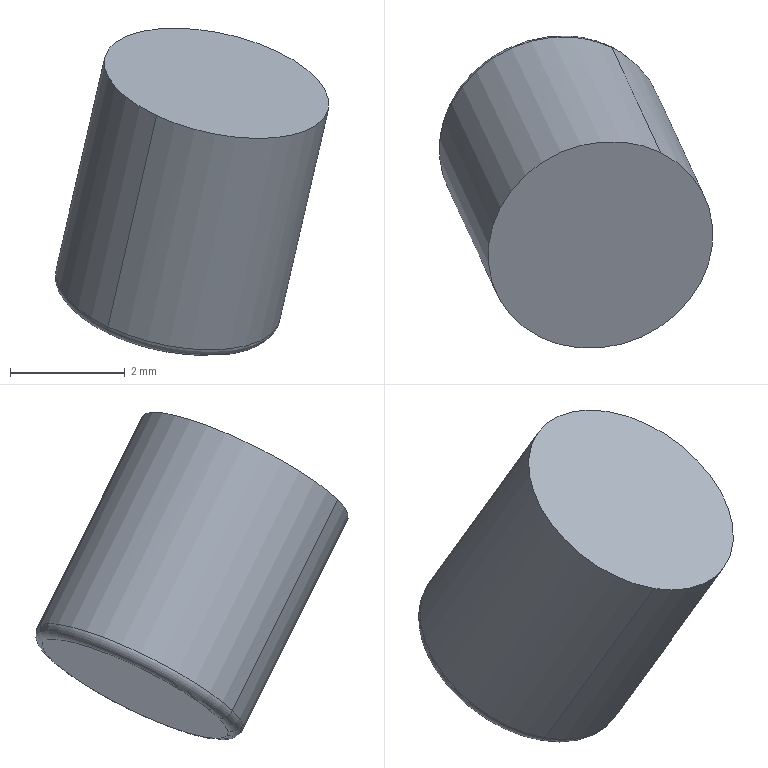Part | SolidWorks | features BaseBody 1 | 1 solid | 8 faces | box 4.768 x 5.451 x 5.709 mm | volume 55.187 mm3 | torus 4 | plane 2 | cylinder 2 | commonest cylinder face diameters 4 x2
STEP:
#1=CARTESIAN_POINT('',(1969.356,-228.956,958.165));
#2=VERTEX_POINT('',#1);
#3=CARTESIAN_POINT('',(1970.758,-225.552,959.535));
#4=VERTEX_POINT('',#3);
#5=CARTESIAN_POINT('',(1970.403,-227.346,958.725));
#6=DIRECTION('',(-0.2015,0.436,-0.8771));
#7=DIRECTION('',(0.9077,0.4197,0.0001618));
#8=AXIS2_PLACEMENT_3D('',#5,#6,#7);
#9=CIRCLE('',#8,2.);
#10=EDGE_CURVE('',#2,#4,#9,.T.);
#11=ORIENTED_EDGE('',*,*,#10,.T.);
#12=CARTESIAN_POINT('',(1970.682,-225.644,959.279));
#13=VERTEX_POINT('',#12);
#14=CARTESIAN_POINT('',(1970.722,-225.731,959.454));
#15=DIRECTION('',(-0.9633,0.07416,0.2581));
#16=DIRECTION('',(0.2588,0.,0.9659));
#17=AXIS2_PLACEMENT_3D('',#14,#15,#16);
#18=CIRCLE('',#17,0.2);
#19=EDGE_CURVE('',#4,#13,#18,.T.);
#20=ORIENTED_EDGE('',*,*,#19,.T.);
#21=CARTESIAN_POINT('',(1969.421,-228.708,958.046));
#22=VERTEX_POINT('',#21);
#23=CARTESIAN_POINT('',(1970.362,-227.259,958.55));
#24=DIRECTION('',(-0.2015,0.436,-0.8771));
#25=DIRECTION('',(0.9077,0.4197,0.0001618));
#26=AXIS2_PLACEMENT_3D('',#23,#24,#25);
#27=CIRCLE('',#26,1.8);
#28=EDGE_CURVE('',#22,#13,#27,.T.);
#29=ORIENTED_EDGE('',*,*,#28,.F.);
#30=CARTESIAN_POINT('',(1969.461,-228.795,958.221));
#31=DIRECTION('',(-0.8281,0.4024,0.3903));
#32=DIRECTION('',(0.5231,0.8049,0.28));
#33=AXIS2_PLACEMENT_3D('',#30,#31,#32);
#34=CIRCLE('',#33,0.2);
#35=EDGE_CURVE('',#22,#2,#34,.T.);
#36=ORIENTED_EDGE('',*,*,#35,.T.);
#37=EDGE_LOOP('',(#11,#20,#29,#36));
#38=FACE_OUTER_BOUND('',#37,.T.);
#39=CARTESIAN_POINT('',(1970.403,-227.346,958.725));
#40=DIRECTION('',(-0.2015,0.436,-0.8771));
#41=DIRECTION('',(0.1776,0.8969,0.4051));
#42=AXIS2_PLACEMENT_3D('',#39,#40,#41);
#43=TOROIDAL_SURFACE('',#42,1.8,0.2);
#44=ADVANCED_FACE('',(#38),#43,.T.);
#45=CARTESIAN_POINT('',(1971.447,-225.888,958.982));
#46=VERTEX_POINT('',#45);
#47=CARTESIAN_POINT('',(1971.447,-225.888,958.982));
#48=CARTESIAN_POINT('',(1971.554,-225.955,958.924));
#49=CARTESIAN_POINT('',(1971.654,-226.033,958.863));
#50=CARTESIAN_POINT('',(1971.744,-226.119,958.799));
#51=CARTESIAN_POINT('',(1971.968,-226.387,958.614));
#52=CARTESIAN_POINT('',(1972.101,-226.71,958.423));
#53=CARTESIAN_POINT('',(1972.143,-226.935,958.302));
#54=CARTESIAN_POINT('',(1972.139,-227.417,958.063));
#55=CARTESIAN_POINT('',(1971.947,-227.884,957.875));
#56=CARTESIAN_POINT('',(1971.798,-228.112,957.796));
#57=CARTESIAN_POINT('',(1971.447,-228.481,957.693));
#58=CARTESIAN_POINT('',(1970.995,-228.727,957.674));
#59=CARTESIAN_POINT('',(1970.773,-228.81,957.684));
#60=CARTESIAN_POINT('',(1970.354,-228.9,957.736));
#61=CARTESIAN_POINT('',(1969.938,-228.876,957.843));
#62=CARTESIAN_POINT('',(1969.755,-228.842,957.902));
#63=CARTESIAN_POINT('',(1969.581,-228.785,957.97));
#64=CARTESIAN_POINT('',(1969.421,-228.708,958.046));
#65=B_SPLINE_CURVE_WITH_KNOTS('',5,(#47,#48,#49,#50,#51,#52,#53,#54,#55,#56,#57,#58,#59,#60,#61,#62,#63,#64),.UNSPECIFIED.,.F.,.F.,(6,3,3,3,3,6),(0.0315,0.1548,0.3787,0.6232,0.829,1.),.UNSPECIFIED.);
#66=EDGE_CURVE('',#46,#22,#65,.T.);
#67=ORIENTED_EDGE('',*,*,#66,.F.);
#68=CARTESIAN_POINT('',(1971.607,-225.823,959.205));
#69=VERTEX_POINT('',#68);
#70=CARTESIAN_POINT('',(1971.487,-225.976,959.157));
#71=DIRECTION('',(0.7724,-0.48,-0.416));
#72=DIRECTION('',(0.5278,0.8494,0.));
#73=AXIS2_PLACEMENT_3D('',#70,#71,#72);
#74=CIRCLE('',#73,0.2);
#75=EDGE_CURVE('',#46,#69,#74,.T.);
#76=ORIENTED_EDGE('',*,*,#75,.T.);
#77=CARTESIAN_POINT('',(1970.403,-227.346,958.725));
#78=DIRECTION('',(-0.2015,0.436,-0.8771));
#79=DIRECTION('',(0.9077,0.4197,0.0001618));
#80=AXIS2_PLACEMENT_3D('',#77,#78,#79);
#81=CIRCLE('',#80,2.);
#82=EDGE_CURVE('',#69,#2,#81,.T.);
#83=ORIENTED_EDGE('',*,*,#82,.T.);
#84=ORIENTED_EDGE('',*,*,#35,.F.);
#85=EDGE_LOOP('',(#67,#76,#83,#84));
#86=FACE_OUTER_BOUND('',#85,.T.);
#87=CARTESIAN_POINT('',(1970.403,-227.346,958.725));
#88=DIRECTION('',(0.2015,-0.436,0.8771));
#89=DIRECTION('',(0.6024,0.7613,0.2401));
#90=AXIS2_PLACEMENT_3D('',#87,#88,#89);
#91=TOROIDAL_SURFACE('',#90,1.8,0.2);
#92=ADVANCED_FACE('',(#86),#91,.T.);
#93=CARTESIAN_POINT('',(1972.295,-227.567,962.969));
#94=VERTEX_POINT('',#93);
#95=CARTESIAN_POINT('',(1970.202,-230.787,961.849));
#96=VERTEX_POINT('',#95);
#97=CARTESIAN_POINT('',(1971.249,-229.177,962.409));
#98=DIRECTION('',(-0.2015,0.436,-0.8771));
#99=DIRECTION('',(0.9077,0.4197,0.0001618));
#100=AXIS2_PLACEMENT_3D('',#97,#98,#99);
#101=CIRCLE('',#100,2.);
#102=EDGE_CURVE('',#94,#96,#101,.T.);
#103=ORIENTED_EDGE('',*,*,#102,.F.);
#104=CARTESIAN_POINT('',(1971.249,-229.177,962.409));
#105=DIRECTION('',(-0.2015,0.436,-0.8771));
#106=DIRECTION('',(0.9077,0.4197,0.0001618));
#107=AXIS2_PLACEMENT_3D('',#104,#105,#106);
#108=CIRCLE('',#107,2.);
#109=EDGE_CURVE('',#96,#94,#108,.T.);
#110=ORIENTED_EDGE('',*,*,#109,.F.);
#111=EDGE_LOOP('',(#103,#110));
#112=FACE_OUTER_BOUND('',#111,.T.);
#113=CARTESIAN_POINT('',(1970.445,-224.727,964.806));
#114=DIRECTION('',(-0.2015,0.436,-0.8771));
#115=DIRECTION('',(-0.9077,-0.4197,-0.0001618));
#116=AXIS2_PLACEMENT_3D('',#113,#114,#115);
#117=PLANE('',#116);
#118=ADVANCED_FACE('',(#112),#117,.F.);
#119=CARTESIAN_POINT('',(1971.449,-225.736,959.285));
#120=VERTEX_POINT('',#119);
#121=CARTESIAN_POINT('',(1971.852,-226.608,961.039));
#122=DIRECTION('',(-0.2015,0.436,-0.8771));
#123=VECTOR('',#122,1000.);
#124=LINE('',#121,#123);
#125=EDGE_CURVE('',#94,#120,#124,.T.);
#126=ORIENTED_EDGE('',*,*,#125,.F.);
#127=ORIENTED_EDGE('',*,*,#102,.T.);
#128=CARTESIAN_POINT('',(1969.759,-229.828,959.919));
#129=DIRECTION('',(0.2015,-0.436,0.8771));
#130=VECTOR('',#129,1000.);
#131=LINE('',#128,#130);
#132=EDGE_CURVE('',#2,#96,#131,.T.);
#133=ORIENTED_EDGE('',*,*,#132,.F.);
#134=ORIENTED_EDGE('',*,*,#82,.F.);
#135=CARTESIAN_POINT('',(1970.403,-227.346,958.725));
#136=DIRECTION('',(-0.2015,0.436,-0.8771));
#137=DIRECTION('',(0.9077,0.4197,0.0001618));
#138=AXIS2_PLACEMENT_3D('',#135,#136,#137);
#139=CIRCLE('',#138,2.);
#140=EDGE_CURVE('',#120,#69,#139,.T.);
#141=ORIENTED_EDGE('',*,*,#140,.F.);
#142=EDGE_LOOP('',(#126,#127,#133,#134,#141));
#143=FACE_OUTER_BOUND('',#142,.T.);
#144=CARTESIAN_POINT('',(1970.805,-228.218,960.479));
#145=DIRECTION('',(-0.2015,0.436,-0.8771));
#146=DIRECTION('',(-0.5231,-0.8049,-0.28));
#147=AXIS2_PLACEMENT_3D('',#144,#145,#146);
#148=CYLINDRICAL_SURFACE('',#147,2.);
#149=ADVANCED_FACE('',(#143),#148,.T.);
#150=ORIENTED_EDGE('',*,*,#132,.T.);
#151=ORIENTED_EDGE('',*,*,#109,.T.);
#152=ORIENTED_EDGE('',*,*,#125,.T.);
#153=CARTESIAN_POINT('',(1970.403,-227.346,958.725));
#154=DIRECTION('',(-0.2015,0.436,-0.8771));
#155=DIRECTION('',(0.9077,0.4197,0.0001618));
#156=AXIS2_PLACEMENT_3D('',#153,#154,#155);
#157=CIRCLE('',#156,2.);
#158=EDGE_CURVE('',#4,#120,#157,.T.);
#159=ORIENTED_EDGE('',*,*,#158,.F.);
#160=ORIENTED_EDGE('',*,*,#10,.F.);
#161=EDGE_LOOP('',(#150,#151,#152,#159,#160));
#162=FACE_OUTER_BOUND('',#161,.T.);
#163=CARTESIAN_POINT('',(1970.805,-228.218,960.479));
#164=DIRECTION('',(-0.2015,0.436,-0.8771));
#165=DIRECTION('',(-0.5231,-0.8049,-0.28));
#166=AXIS2_PLACEMENT_3D('',#163,#164,#165);
#167=CYLINDRICAL_SURFACE('',#166,2.);
#168=ADVANCED_FACE('',(#162),#167,.T.);
#169=CARTESIAN_POINT('',(1971.304,-225.81,959.054));
#170=VERTEX_POINT('',#169);
#171=CARTESIAN_POINT('',(1971.304,-225.81,959.054));
#172=CARTESIAN_POINT('',(1971.333,-225.824,959.04));
#173=CARTESIAN_POINT('',(1971.362,-225.839,959.026));
#174=CARTESIAN_POINT('',(1971.391,-225.855,959.011));
#175=CARTESIAN_POINT('',(1971.419,-225.871,958.997));
#176=CARTESIAN_POINT('',(1971.447,-225.888,958.982));
#177=B_SPLINE_CURVE_WITH_KNOTS('',5,(#171,#172,#173,#174,#175,#176),.UNSPECIFIED.,.F.,.F.,(6,6),(0.,0.0315),.UNSPECIFIED.);
#178=EDGE_CURVE('',#170,#46,#177,.T.);
#179=ORIENTED_EDGE('',*,*,#178,.T.);
#180=ORIENTED_EDGE('',*,*,#66,.T.);
#181=ORIENTED_EDGE('',*,*,#28,.T.);
#182=CARTESIAN_POINT('',(1970.362,-227.259,958.55));
#183=DIRECTION('',(-0.2015,0.436,-0.8771));
#184=DIRECTION('',(0.9077,0.4197,0.0001618));
#185=AXIS2_PLACEMENT_3D('',#182,#183,#184);
#186=CIRCLE('',#185,1.8);
#187=EDGE_CURVE('',#13,#170,#186,.T.);
#188=ORIENTED_EDGE('',*,*,#187,.T.);
#189=EDGE_LOOP('',(#179,#180,#181,#188));
#190=FACE_OUTER_BOUND('',#189,.T.);
#191=CARTESIAN_POINT('',(1969.559,-222.808,960.947));
#192=DIRECTION('',(-0.2015,0.436,-0.8771));
#193=DIRECTION('',(-0.9077,-0.4197,-0.0001618));
#194=AXIS2_PLACEMENT_3D('',#191,#192,#193);
#195=PLANE('',#194);
#196=ADVANCED_FACE('',(#190),#195,.T.);
#197=ORIENTED_EDGE('',*,*,#75,.F.);
#198=ORIENTED_EDGE('',*,*,#178,.F.);
#199=CARTESIAN_POINT('',(1971.344,-225.897,959.229));
#200=DIRECTION('',(-0.8281,0.4024,0.3903));
#201=DIRECTION('',(0.5231,0.8049,0.28));
#202=AXIS2_PLACEMENT_3D('',#199,#200,#201);
#203=CIRCLE('',#202,0.2);
#204=EDGE_CURVE('',#120,#170,#203,.T.);
#205=ORIENTED_EDGE('',*,*,#204,.F.);
#206=ORIENTED_EDGE('',*,*,#140,.T.);
#207=EDGE_LOOP('',(#197,#198,#205,#206));
#208=FACE_OUTER_BOUND('',#207,.T.);
#209=CARTESIAN_POINT('',(1970.403,-227.346,958.725));
#210=DIRECTION('',(0.2015,-0.436,0.8771));
#211=DIRECTION('',(0.6024,0.7613,0.2401));
#212=AXIS2_PLACEMENT_3D('',#209,#210,#211);
#213=TOROIDAL_SURFACE('',#212,1.8,0.2);
#214=ADVANCED_FACE('',(#208),#213,.T.);
#215=ORIENTED_EDGE('',*,*,#19,.F.);
#216=ORIENTED_EDGE('',*,*,#158,.T.);
#217=ORIENTED_EDGE('',*,*,#204,.T.);
#218=ORIENTED_EDGE('',*,*,#187,.F.);
#219=EDGE_LOOP('',(#215,#216,#217,#218));
#220=FACE_OUTER_BOUND('',#219,.T.);
#221=CARTESIAN_POINT('',(1970.403,-227.346,958.725));
#222=DIRECTION('',(-0.2015,0.436,-0.8771));
#223=DIRECTION('',(0.1776,0.8969,0.4051));
#224=AXIS2_PLACEMENT_3D('',#221,#222,#223);
#225=TOROIDAL_SURFACE('',#224,1.8,0.2);
#226=ADVANCED_FACE('',(#220),#225,.T.);
#227=CLOSED_SHELL('',(#44,#92,#118,#149,#168,#196,#214,#226));
#228=MANIFOLD_SOLID_BREP('',#227);
#229=CARTESIAN_POINT('',(0.,0.,0.));
#230=DIRECTION('',(0.,0.,1.));
#231=DIRECTION('',(1.,0.,0.));
#232=AXIS2_PLACEMENT_3D('',#229,#230,#231);
#233=(LENGTH_UNIT()NAMED_UNIT(*)SI_UNIT(.MILLI.,.METRE.));
#234=UNCERTAINTY_MEASURE_WITH_UNIT(LENGTH_MEASURE(0.00001),#233,'','');
#235=(NAMED_UNIT(*)PLANE_ANGLE_UNIT()SI_UNIT($,.RADIAN.));
#236=(NAMED_UNIT(*)SI_UNIT($,.STERADIAN.)SOLID_ANGLE_UNIT());
#237=(GEOMETRIC_REPRESENTATION_CONTEXT(3)GLOBAL_UNCERTAINTY_ASSIGNED_CONTEXT((#234))GLOBAL_UNIT_ASSIGNED_CONTEXT((#233,#235,#236))REPRESENTATION_CONTEXT('',''));
#238=ADVANCED_BREP_SHAPE_REPRESENTATION('',(#228,#232),#237);